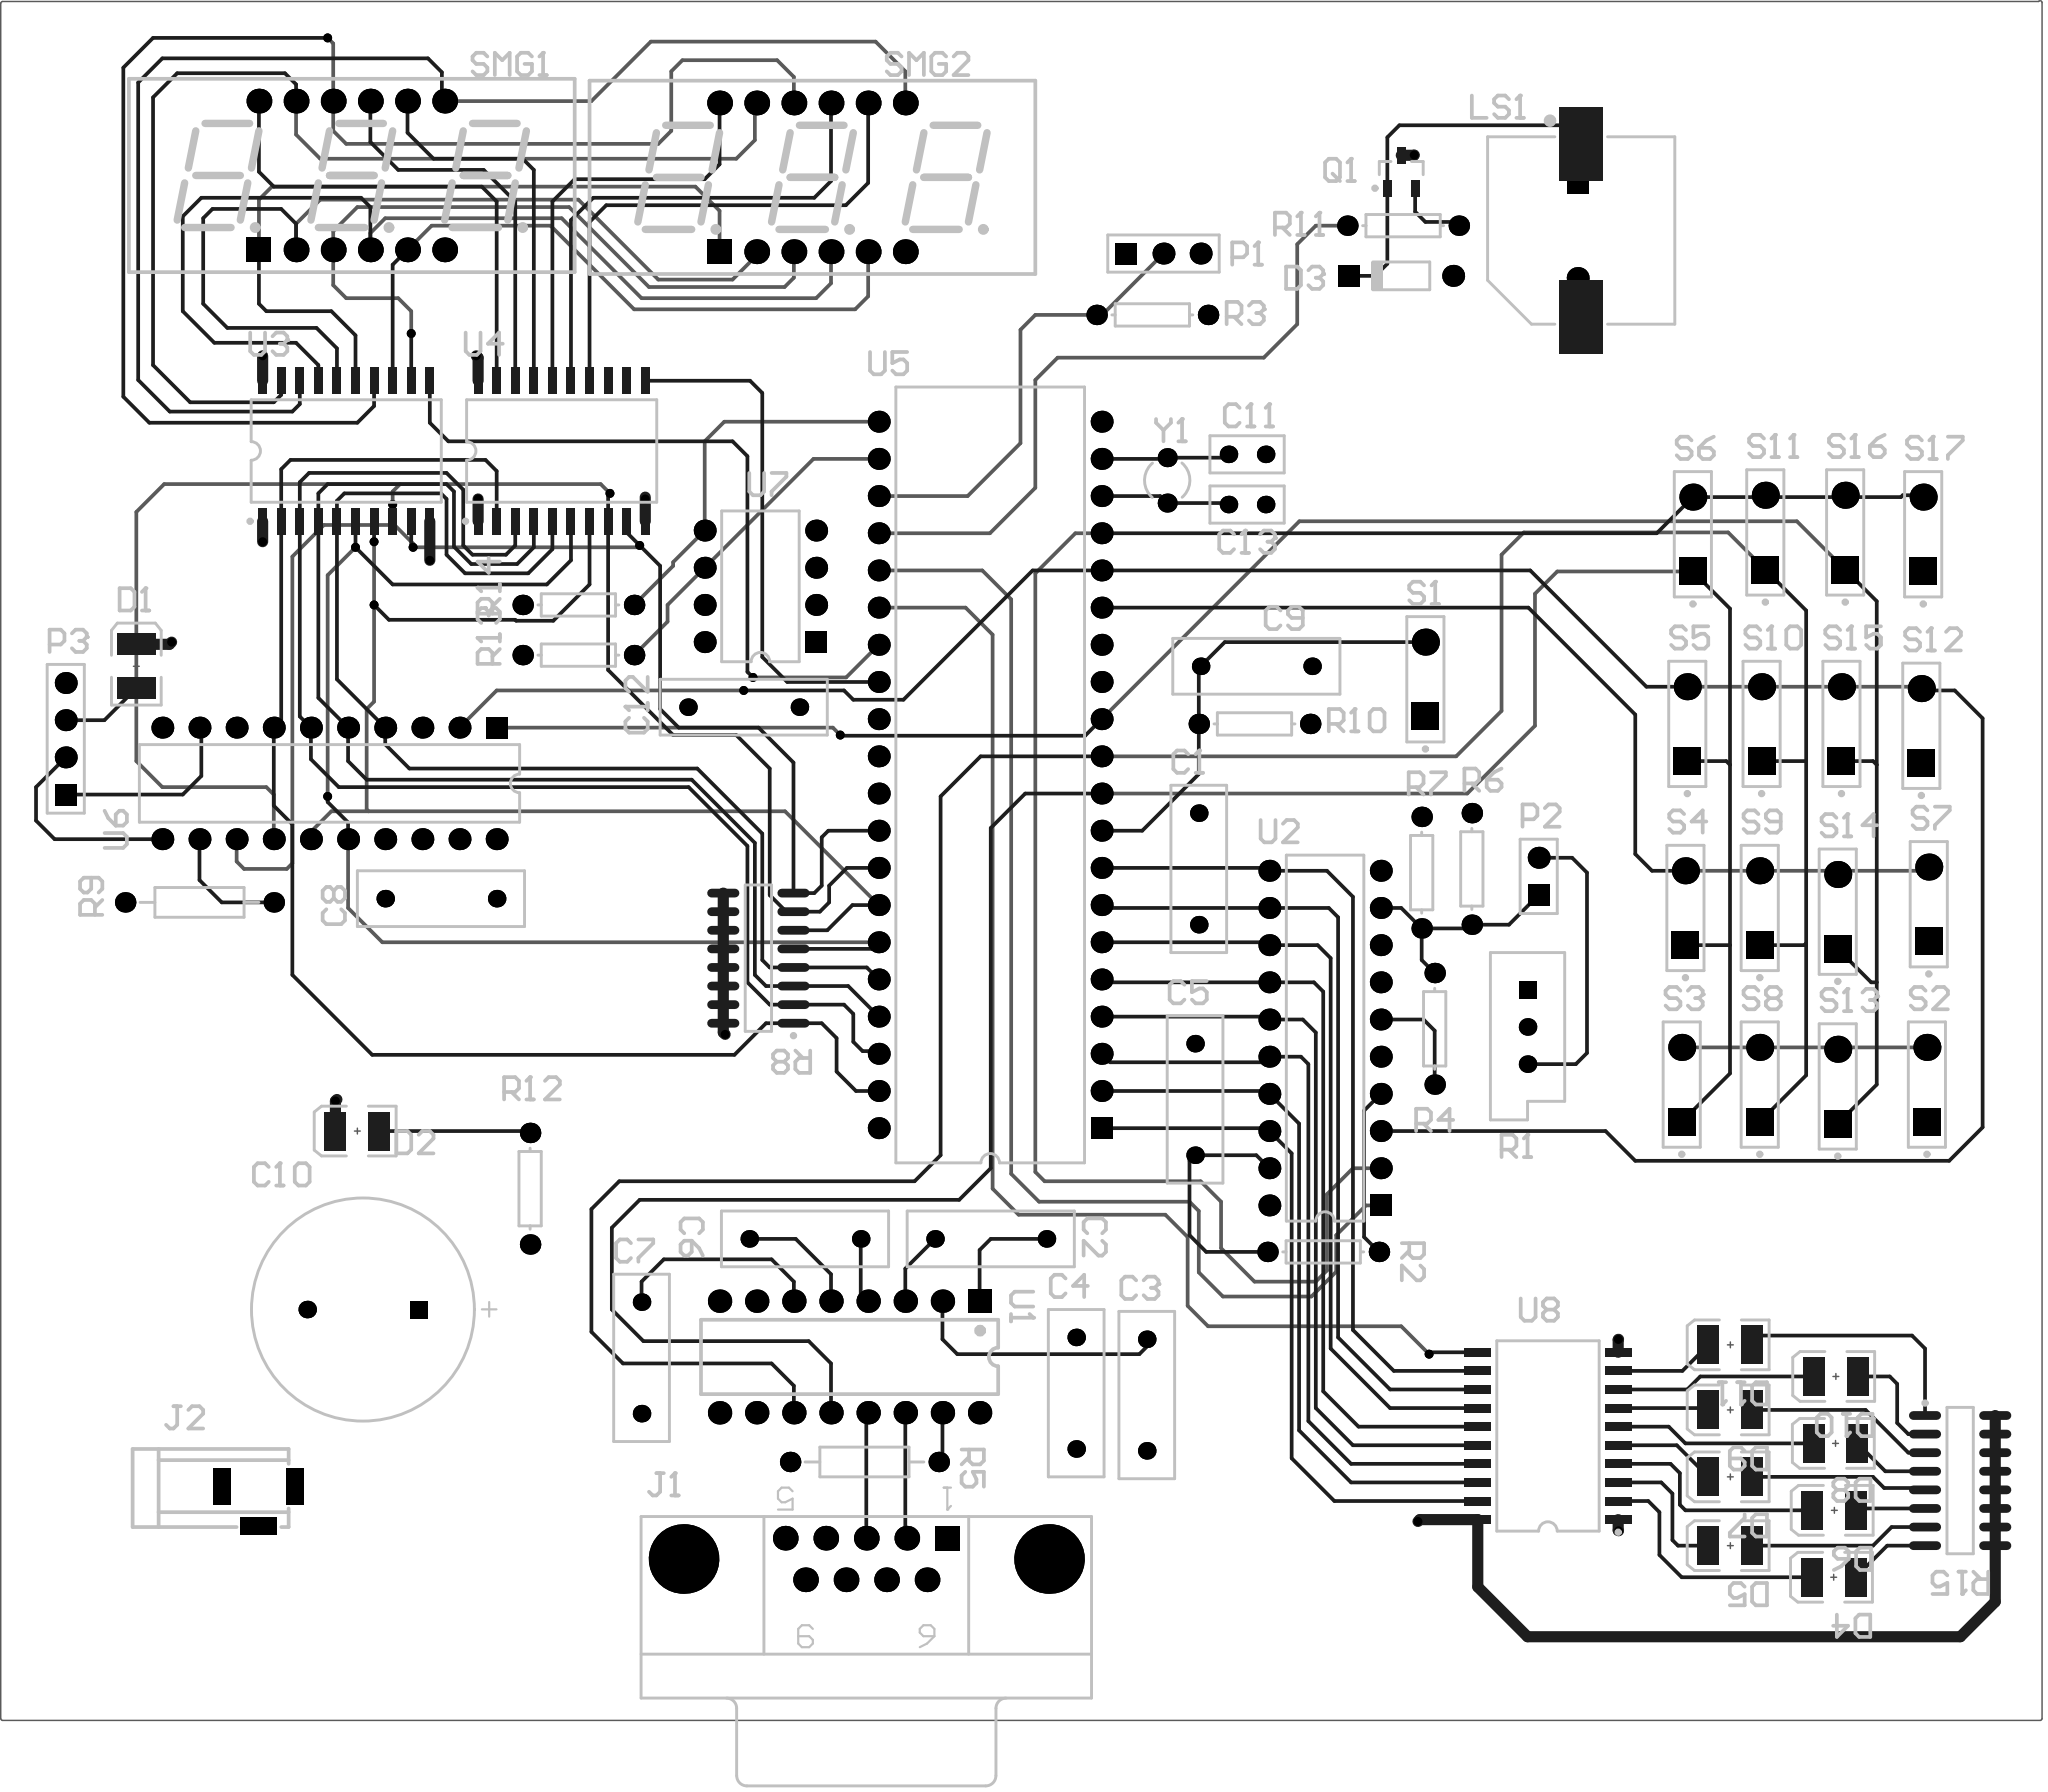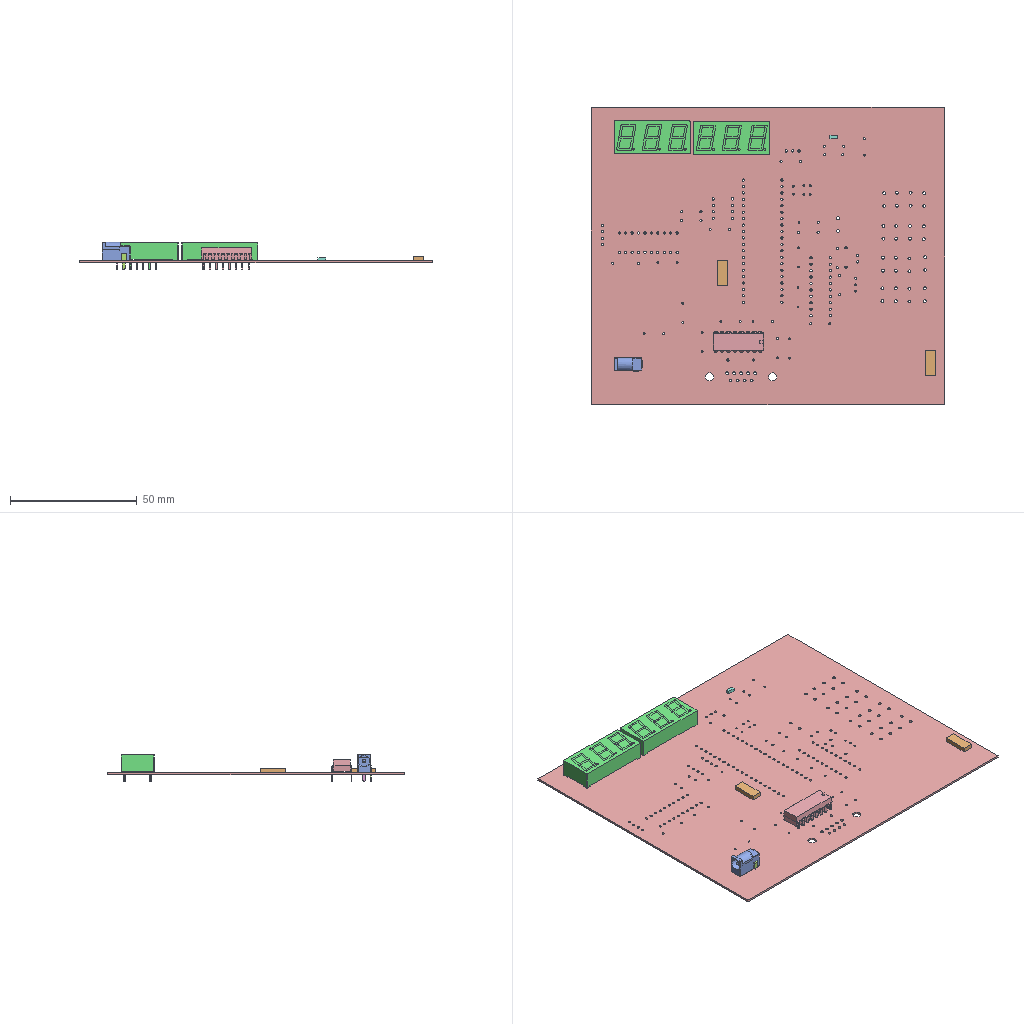Circuit board layout | Altium Designer | box 139.6 x 117.5 x 10.9 mm
Layer stack:
# Altium Designer layer stack of  (unit mm; dielectric type: 0 none, 1 core, 2 prepreg, 3 surface material)
index,name,kind,layer,copper_thickness_mm,dielectric_type,dielectric_thickness_mm,dielectric_material,dielectric_constant
0,Top Paste,other,,,,,,
1,Top Overlay,other,,,,,,
2,Top Solder,dielectric,,,3,0.0102,Solder Resist,3.5
3,Top Layer,copper,Top Layer,0.0356,,,,
4,Dielectric 1,dielectric,,,1,0.254,FR-4,4.2
5,VCC,copper,VCC,0.036,,,,
6,Dielectric 3,dielectric,,,2,0.127,,4.2
7,GND,copper,GND,0.036,,,,
8,Dielectric 2,dielectric,,,1,0.254,,4.2
9,Bottom Layer,copper,Bottom Layer,0.0356,,,,
10,Bottom Solder,dielectric,,,3,0.0102,Solder Resist,3.5
11,Bottom Overlay,other,,,,,,
12,Bottom Paste,other,,,,,,
# drill layer pairs: low layer,high layer
drill_pair,Top Layer,Bottom Layer
Part placement:
Designator,Comment,Layer,Footprint,Center-X(mm),Center-Y(mm),Rotation
C1,104,TopLayer,RAD-0.3,98.298,83.185,90
C2,104,TopLayer,RAD-0.3,84.074,57.912,180
C3,104,TopLayer,RAD-0.3,94.742,47.244,90
C4,104,TopLayer,RAD-0.3,89.916,47.371,90
C5,104,TopLayer,RAD-0.3,98.044,67.437,90
C6,104,TopLayer,RAD-0.3,71.374,57.912,180
C7,104,TopLayer,RAD-0.3,60.198,49.784,90
C8,104,TopLayer,RAD-0.3,46.482,81.153,180
C9,10UF,TopLayer,RAD-0.3,102.235,97.028,360
C10,100UF,TopLayer,RB7.6-15,41.148,53.086,0
C11,20PF,TopLayer,RAD-0.1,101.6,111.506,360
C12,104,TopLayer,RAD-0.3,67.183,94.234,180
C13,20PF,TopLayer,RAD-0.1,101.6,108.077,360
D1,LED3,TopLayer,3.5X2.8X1.9,25.654,97.028,90
D2,LED3,TopLayer,3.5X2.8X1.9,40.767,65.278,180
D3,Diode 1N4148,TopLayer,DO-35,112.141,123.698,180
D4,LED3,TopLayer,3.5X2.8X1.9,141.708,34.798,180
D5,LED3,TopLayer,3.5X2.8X1.9,134.644,36.957,180
D6,LED3,TopLayer,3.5X2.8X1.9,141.756,39.37,180
D7,LED3,TopLayer,3.5X2.8X1.9,134.644,41.656,180
D8,LED3,TopLayer,3.5X2.8X1.9,141.835,43.942,180
D9,LED3,TopLayer,3.5X2.8X1.9,134.644,46.228,180
D10,LED3,TopLayer,3.5X2.8X1.9,141.859,48.514,180
D11,LED3,TopLayer,3.5X2.8X1.9,134.644,50.673,180
J1,D Connector 9,TopLayer,DSUB1.385-2H9,75.565,36.045,180
J2,PWR2.5,TopLayer,DC-002,33.996,39.671,180
LS1,Buzzer,TopLayer,ABSM-1574,124.326,126.798,270
P1,DS18B20,TopLayer,HDR1X3,95.885,125.222,360
P2,Header 2,TopLayer,HDR1X2,121.539,82.677,90
P3,Header 4,TopLayer,HDR1X4,20.828,92.075,90
Q1,PNP,TopLayer,SOT-23B_N,112.141,130.81,90
R1,RPot,TopLayer,VR5,120.777,72.39,270
R2,10K,TopLayer,AXIAL-0.3,106.807,57.023,360
R3,4.7K,TopLayer,AXIAL-0.3,95.123,121.031,360
R4,10K,TopLayer,AXIAL-0.3,114.427,72.263,270
R5,0,TopLayer,AXIAL-0.4,75.438,42.672,360
R6,1k,TopLayer,AXIAL-0.3,116.967,83.185,270
R7,1K,TopLayer,AXIAL-0.3,113.538,82.931,90
R8,Res Pack3,TopLayer,SO-16_N,68.186,77.089,180
R9,0,TopLayer,AXIAL-0.4,29.972,80.899,180
R10,10K,TopLayer,AXIAL-0.3,102.108,93.091,180
R11,2K,TopLayer,AXIAL-0.3,112.268,127.127,180
R12,2K,TopLayer,AXIAL-0.3,52.578,61.341,270
R13,4.7K,TopLayer,AXIAL-0.3,55.88,97.79,180
R14,4.7K,TopLayer,AXIAL-0.3,55.88,101.219,180
R15,Res Pack3,TopLayer,SO-16_N,150.355,41.402,360
S1,SW-PB,TopLayer,SPST-2,113.792,96.139,90
S2,SW-PB,TopLayer,SPST-2,148.082,68.453,90
S3,SW-PB,TopLayer,SPST-2,131.318,68.453,90
S4,SW-PB,TopLayer,SPST-2,131.572,80.518,90
S5,SW-PB,TopLayer,SPST-2,131.699,93.091,90
S6,SW-PB,TopLayer,SPST-2,132.08,106.045,90
S7,SW-PB,TopLayer,SPST-2,148.209,80.772,90
S8,SW-PB,TopLayer,SPST-2,136.652,68.453,90
S9,SW-PB,TopLayer,SPST-2,136.652,80.518,90
S10,SW-PB,TopLayer,SPST-2,136.779,93.091,90
S11,SW-PB,TopLayer,SPST-2,137.033,106.172,90
S12,SW-PB,TopLayer,SPST-2,147.701,92.964,90
S13,SW-PB,TopLayer,SPST-2,141.986,68.326,90
S14,SW-PB,TopLayer,SPST-2,141.986,80.264,90
S15,SW-PB,TopLayer,SPST-2,142.24,93.091,90
S16,SW-PB,TopLayer,SPST-2,142.494,106.172,90
S17,SW-PB,TopLayer,SPST-2,147.828,106.045,90
SMG1,3931A,TopLayer,SMG_0.39-3P,40.386,130.556,360
SMG2,3931A,TopLayer,SMG_0.39-3P,71.882,130.429,360
U1,MAX232ESE,TopLayer,DIP16,74.422,49.844,270
U2,ADC0804CN,TopLayer,N020,106.934,71.628,90
U3,MC74HC573DW,TopLayer,751D-03,40.005,111.734,0
U4,MC74HC573DW,TopLayer,751D-03,54.737,111.734,0
U5,P89C51RC2HBP,TopLayer,SOT129-1,84.037,89.605,90
U6,DAC0832LCJ,TopLayer,J20A,38.862,89.027,180
U7,M24C02BN6,TopLayer,PSDIP8A,68.326,102.489,90
U8,MC74HC573ADW,TopLayer,751D-05,122.174,44.45,90
Y1,XTAL,TopLayer,R38,96.139,109.728,180
Pad and via stacks:
# Altium Designer via and pad stacks of  (unit mm). Each distinct definition once, with the count of objects using it.
# via: kind,start_layer,end_layer,hole_mm,diameter_mm,mode(0 simple;1 top-mid-bottom;2 full stack),diameter_per_layer,count,example_net
# pad: kind,layer,hole_mm,hole_type(0 round;1 square;2 slot),plating,top_size,top_shape(1 round;2 rect;3 octagon;9 rounded rect),mid_size,bottom_size,mode,footprint,size_per_layer,count,example
pad,Multi-Layer,1.1,0,plated,1.85x1.85,1,1.85x1.85,1.85x1.85,0,SPST-2,,17,S13.2
pad,Multi-Layer,1.1,0,plated,1.85x1.85,2,1.85x1.85,1.85x1.85,0,SPST-2,,17,S13.1
pad,Multi-Layer,0.7,0,plated,1.2x1.2,1,1.2x1.2,1.2x1.2,0,RAD-0.1,,4,C13.2
pad,Multi-Layer,0.85,0,plated,1.4x1.4,1,1.4x1.4,1.4x1.4,0,AXIAL-0.3,,20,R13.1
pad,Multi-Layer,0.7,0,plated,1.3x1.3,1,1.3x1.3,1.3x1.3,0,R38,,2,Y1.2
pad,Multi-Layer,0.9,0,plated,1.5x1.5,1,1.5x1.5,1.5x1.5,0,PSDIP8A,,7,U7.5
pad,Multi-Layer,0.9,0,plated,1.5x1.5,2,1.5x1.5,1.5x1.5,0,PSDIP8A,,1,U7.1
pad,Multi-Layer,0.9,0,plated,1.5x1.5,1,1.5x1.5,1.5x1.5,0,DO-35,,1,D3.1
pad,Multi-Layer,0.9,0,plated,1.5x1.5,2,1.5x1.5,1.5x1.5,0,DO-35,,1,D3.2
pad,Multi-Layer,0.7,0,plated,1.2x1.2,1,1.2x1.2,1.2x1.2,0,RAD-0.3,,20,C12.1
pad,Multi-Layer,0.7,0,plated,1.5x1.5,1,1.5x1.5,1.5x1.5,0,ABSM-1574,,1,LS1.2A
pad,Multi-Layer,0.7,0,plated,1.5x1.5,2,1.5x1.5,1.5x1.5,0,ABSM-1574,,1,LS1.1A
pad,Multi-Layer,0.7,0,plated,1.2x1.2,1,1.2x1.2,1.2x1.2,0,RB7.6-15,,1,C10.2
pad,Multi-Layer,0.7,0,plated,1.2x1.2,2,1.2x1.2,1.2x1.2,0,RB7.6-15,,1,C10.1
pad,Multi-Layer,0.6,2,plated,2.5x1.2,2,2.5x1.2,2.5x1.2,0,DC-002,,3,J2.1
pad,Multi-Layer,0.85,0,plated,1.4x1.4,1,1.4x1.4,1.4x1.4,0,AXIAL-0.4,,4,R9.2
pad,Multi-Layer,0.8,0,plated,1.7x1.7,1,1.7x1.7,1.7x1.7,0,SMG 0.39-3P,,22,SMG1.6
pad,Multi-Layer,0.8,0,plated,1.7x1.7,2,1.7x1.7,1.7x1.7,0,SMG 0.39-3P,,2,SMG1.1
pad,Multi-Layer,0.9,0,plated,1.5x1.5,2,1.5x1.5,1.5x1.5,0,J20A,,1,U6.1
pad,Multi-Layer,0.9,0,plated,1.5x1.5,1,1.5x1.5,1.5x1.5,0,J20A,,19,U6.2
pad,Multi-Layer,0.9,0,plated,1.5x1.5,2,1.5x1.5,1.5x1.5,0,HDR1X4,,1,P3.1
pad,Multi-Layer,0.9,0,plated,1.5x1.5,1,1.5x1.5,1.5x1.5,0,HDR1X4,,3,P3.2
pad,Multi-Layer,0.9,0,plated,1.5x1.5,2,1.5x1.5,1.5x1.5,0,SOT129-1,,1,U5.1
pad,Multi-Layer,0.9,0,plated,1.5x1.5,1,1.5x1.5,1.5x1.5,0,SOT129-1,,39,U5.2
pad,Multi-Layer,0.9,0,plated,1.5x1.5,1,1.5x1.5,1.5x1.5,0,HDR1X2,,1,P2.2
pad,Multi-Layer,0.9,0,plated,1.5x1.5,2,1.5x1.5,1.5x1.5,0,HDR1X2,,1,P2.1
pad,Multi-Layer,0.9,0,plated,1.5x1.5,1,1.5x1.5,1.5x1.5,0,HDR1X3,,2,P1.3
pad,Multi-Layer,0.9,0,plated,1.5x1.5,2,1.5x1.5,1.5x1.5,0,HDR1X3,,1,P1.1
pad,Multi-Layer,1.09,0,plated,1.69x1.69,1,1.69x1.69,1.69x1.69,0,DSUB1.385-2H9,,8,J1.5
pad,Multi-Layer,1.09,0,plated,1.69x1.69,2,1.69x1.69,1.69x1.69,0,DSUB1.385-2H9,,1,J1.1
pad,Multi-Layer,3.26,0,plated,4.76x4.76,1,4.76x4.76,4.76x4.76,0,DSUB1.385-2H9,,2,J1.10
pad,Multi-Layer,0.9,0,plated,1.5x1.5,2,1.5x1.5,1.5x1.5,0,N020,,1,U2.1
pad,Multi-Layer,0.9,0,plated,1.5x1.5,1,1.5x1.5,1.5x1.5,0,N020,,19,U2.2
pad,Multi-Layer,0.7,0,plated,1.2x1.2,1,1.2x1.2,1.2x1.2,0,VR5,,2,R1.3
pad,Multi-Layer,0.7,0,plated,1.2x1.2,2,1.2x1.2,1.2x1.2,0,VR5,,1,R1.1
pad,Multi-Layer,0.8128,0,plated,1.6x1.6,1,1.6x1.6,1.6x1.6,0,DIP16,,15,U1.16
pad,Multi-Layer,0.8128,0,plated,1.6x1.6,2,1.6x1.6,1.6x1.6,0,DIP16,,1,U1.1
pad,Top Layer,0,0,plated,1.5x2.6,2,1.5x2.6,1.5x2.6,0,3.5X2.8X1.9,,20,D11.1
pad,Top Layer,0,0,plated,0.6x2.2,1,0.6x2.2,0.6x2.2,0,SO-16_N,,32,R15.9
pad,Top Layer,0,0,plated,1.8x0.6,2,1.8x0.6,1.8x0.6,0,751D-05,,20,U8.1
pad,Top Layer,0,0,plated,3x5,2,3x5,3x5,0,ABSM-1574,,2,LS1.2
pad,Top Layer,0,0,plated,0.6x1.15,2,0.6x1.15,0.6x1.15,0,SOT-23B_N,,3,Q1.3
pad,Top Layer,0,0,plated,1.8x0.6,2,1.8x0.6,1.8x0.6,0,751D-03,,40,U3.1
via,Top Layer,Bottom Layer,0.3048,0.6096,0,,27,GND
Design rules, without the lines most boards share:
# Altium Designer design rules of  (exported by Altium Designer, unit mm)
# columns: name | kind | enabled | priority | scope1 | scope2 | descriptor | typed fields (field=value)
Clearance | 0 | enabled | 1 | All | All | Clearance Constraint (Gap=10mil) (All),(All) | gap=0.254
PlaneConnect | 6 | enabled | 1 | All | All | Power Plane Connect Rule(Relief Connect )(Expansion=20mil) (Conductor Width=10mil) (Air Gap=10mil) (Entries=4) (All) | relief_conductor_width=0.254 relief_entries=4 relief_expansion=0.508
PolygonConnect | 20 | enabled | 1 | All | All | Polygon Connect Rule(Relief Connect )(Conductor Width=10mil) (Relief Angle=90 Angle) (Entries=4) (Air Gap Width=10mil) (All),(All) | connect_style(0=relief,1=direct,2=none)=0 relief_conductor_width=0.254 relief_entries=4
Width | 2 | enabled | 1 | All | All | Width Constraint (Min=10mil) (Max=30mil) (Preferred=10mil) (All) |
RoutingVias | 11 | enabled | 1 | All | All | Routing Via (MinHoleWidth=28mil) (MaxHoleWidth=28mil) (PreferredHoleWidth=28mil) (MinWidth=50mil) (MaxWidth=50mil) (PreferedWidth=50mil) (All) | via_min_hole=0.7112 via_max_hole=0.7112 via_preferred_diameter=1.27 via_preferred_hole=0.7112
SolderMaskExpansion | 13 | enabled | 1 | All | All | Solder Mask Expansion (Expansion =4mil) (All) | expansion=0.1016
HoleSize | 42 | enabled | 1 | All | All | Hole Size Constraint (Min=1mil) (Max=10000mil) (All) |
DiffPairsRouting | 51 | enabled | 1 | All | All | Differential Pairs Uncoupled Length using the Gap Constraints (Min=10mil) (Max=10mil) (Prefered=10mil)  and Width Constraints (Min=15mil) (Max=15mil) (Prefered=15mil) (All) |
HoleToHoleClearance | 52 | enabled | 1 | All | All | Hole To Hole Clearance (Gap=10mil) (All),(All) | gap=0.254
MinimumSolderMaskSliver | 53 | enabled | 1 | All | All | Minimum Solder Mask Sliver (Gap=0mil) (All),(All) |
SilkToSolderMaskClearance | 54 | enabled | 1 | IsPad | All | Silk To Solder Mask (Clearance=0mil) (IsPad),(All) |
SilkToSilkClearance | 55 | enabled | 1 | All | All | Silk to Silk (Clearance=0mil) (All),(All) |
Classes set for this board:
# Altium Designer classes of  (member kind: 0 net, 1 component, 2 from-to, 3 pad, 4 layer, 5 differential pair, 6 design channel, 7 polygon, 8 structure, 9 xSignal)
# columns: class name | member kind | superclass | members
Sheet1 | 1 | no | C1; C2; C3; C4; C5; C6; C7; C8; C9; C10; C11; C12; C13; D1; D2; D3; D4; D5; D6; D7; D8; D9; D10; D11; J1; J2; LS1; P1; P2; P3; Q1; R1; R2; R3; R4; R5; R6; R7; R8; R9; R10; R11; R12; R13; R14; R15; S1; S2; S3; S4; S5; S6; S7; S8; S9; S10; S11; S12; S13; S14; S15; S16; S17; SMG1; SMG2; U1; U2; U3; U4; U5; U6; U7; U8; Y1;